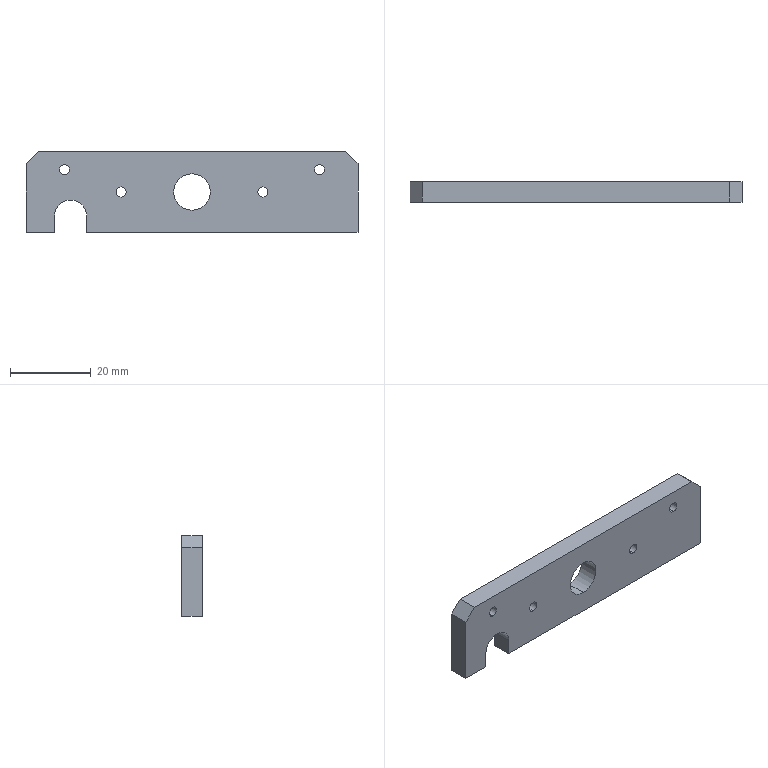Part | STEP file | Load cell connecting block V1.201001 | 1 solid | 23 faces | box 82 x 5 x 20 mm | volume 7453 mm3 | cylinder 12 | plane 11 | commonest cylinder face diameters 2.5 x8 8 x2 9 x2